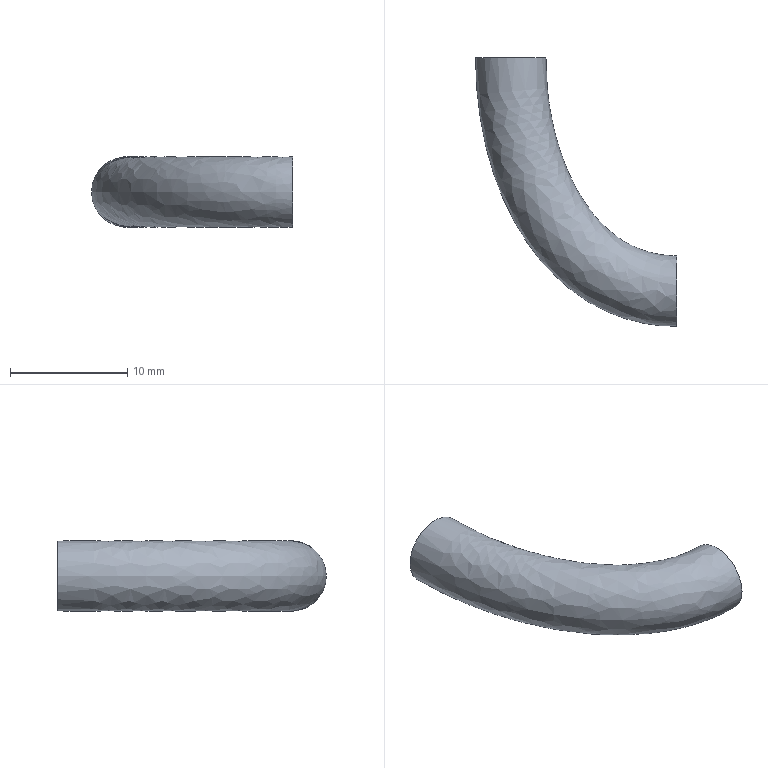Part | NX | features solid 2 | 1 solid | 4 faces | box 17.132 x 22.886 x 6 mm | volume 425.181 mm3 | plane 2 | spline 2